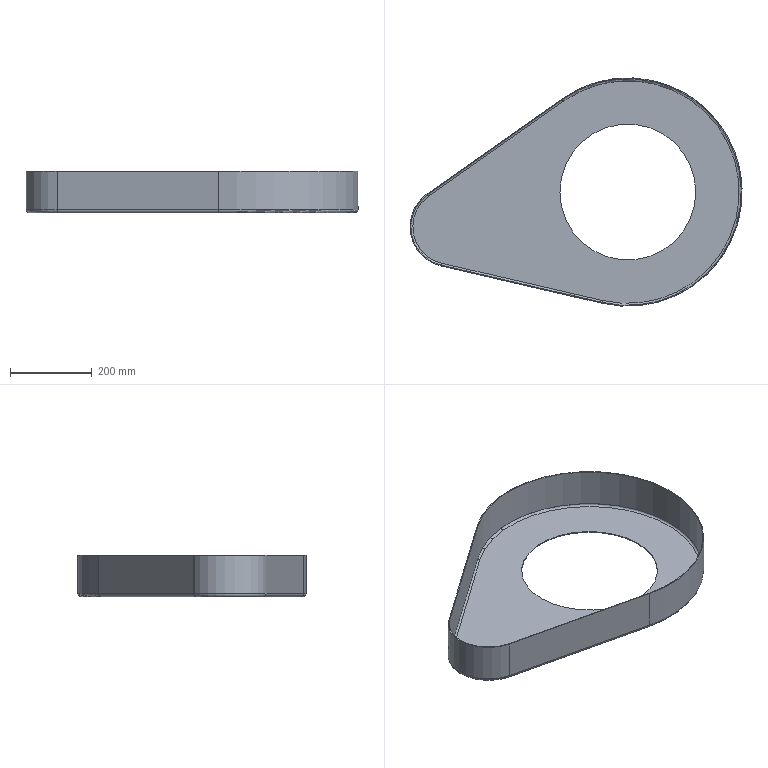Part | Creo | features DATUM PLANE 3, CURVE 2, PROTRUSION 2, ROUND 2, COORDINATE SYSTEM 1 | 1 solid | 21 faces | box 814.237 x 560 x 102 mm | volume 885224 mm3 | cylinder 10 | plane 7 | torus 4 | commonest cylinder face diameters 10 x2 14 x2 333.235 x2 193.453 x1 197.453 x1 556 x1
STEP:
#1=CARTESIAN_POINT('',(0.,0.,0.));
#2=DIRECTION('',(0.,0.,1.));
#3=DIRECTION('',(1.,0.,0.));
#4=AXIS2_PLACEMENT_3D('',#1,#2,#3);
#5=CARTESIAN_POINT('',(-50.882,-259.323,0.));
#6=VERTEX_POINT('',#5);
#7=CARTESIAN_POINT('',(-445.479,-167.904,0.));
#8=VERTEX_POINT('',#7);
#9=CARTESIAN_POINT('',(-50.882,-259.323,0.));
#10=DIRECTION('',(-0.9742,0.2257,0.));
#11=VECTOR('',#10,405.048);
#12=LINE('',#9,#11);
#13=EDGE_CURVE('',#6,#8,#12,.T.);
#14=ORIENTED_EDGE('',*,*,#13,.F.);
#15=CARTESIAN_POINT('',(-146.54,229.778,0.));
#16=VERTEX_POINT('',#15);
#17=CARTESIAN_POINT('',(10.734,6.632,0.));
#18=DIRECTION('',(0.,0.,-1.));
#19=DIRECTION('',(-0.5761,0.8174,0.));
#20=AXIS2_PLACEMENT_3D('',#17,#18,#19);
#21=CIRCLE('',#20,273.);
#22=EDGE_CURVE('',#16,#6,#21,.T.);
#23=ORIENTED_EDGE('',*,*,#22,.F.);
#24=CARTESIAN_POINT('',(-477.619,-3.568,0.));
#25=VERTEX_POINT('',#24);
#26=CARTESIAN_POINT('',(-477.619,-3.568,0.));
#27=DIRECTION('',(0.8174,0.5761,0.));
#28=VECTOR('',#27,405.048);
#29=LINE('',#26,#28);
#30=EDGE_CURVE('',#25,#16,#29,.T.);
#31=ORIENTED_EDGE('',*,*,#30,.F.);
#32=CARTESIAN_POINT('',(-424.776,-78.544,0.));
#33=DIRECTION('',(0.,0.,-1.));
#34=DIRECTION('',(-0.2257,-0.9742,0.));
#35=AXIS2_PLACEMENT_3D('',#32,#33,#34);
#36=CIRCLE('',#35,91.727);
#37=EDGE_CURVE('',#8,#25,#36,.T.);
#38=ORIENTED_EDGE('',*,*,#37,.F.);
#39=EDGE_LOOP('',(#14,#23,#31,#38));
#40=FACE_OUTER_BOUND('',#39,.F.);
#41=CARTESIAN_POINT('',(177.351,6.632,0.));
#42=VERTEX_POINT('',#41);
#43=CARTESIAN_POINT('',(-155.883,6.632,0.));
#44=VERTEX_POINT('',#43);
#45=CARTESIAN_POINT('',(10.734,6.632,0.));
#46=DIRECTION('',(0.,0.,-1.));
#47=DIRECTION('',(1.,0.,0.));
#48=AXIS2_PLACEMENT_3D('',#45,#46,#47);
#49=CIRCLE('',#48,166.617);
#50=EDGE_CURVE('',#42,#44,#49,.T.);
#51=ORIENTED_EDGE('',*,*,#50,.T.);
#52=CARTESIAN_POINT('',(10.734,6.632,0.));
#53=DIRECTION('',(0.,0.,-1.));
#54=DIRECTION('',(-1.,0.,0.));
#55=AXIS2_PLACEMENT_3D('',#52,#53,#54);
#56=CIRCLE('',#55,166.617);
#57=EDGE_CURVE('',#44,#42,#56,.T.);
#58=ORIENTED_EDGE('',*,*,#57,.T.);
#59=EDGE_LOOP('',(#51,#58));
#60=FACE_BOUND('',#59,.F.);
#61=CARTESIAN_POINT('',(0.,0.,0.));
#62=DIRECTION('',(0.,0.,1.));
#63=DIRECTION('',(1.,0.,0.));
#64=AXIS2_PLACEMENT_3D('',#61,#62,#63);
#65=PLANE('',#64);
#66=ADVANCED_FACE('',(#40,#60),#65,.F.);
#67=ORIENTED_EDGE('',*,*,#50,.F.);
#68=CARTESIAN_POINT('',(177.351,6.632,2.));
#69=VERTEX_POINT('',#68);
#70=CARTESIAN_POINT('',(177.351,6.632,0.));
#71=DIRECTION('',(0.,0.,1.));
#72=VECTOR('',#71,2.);
#73=LINE('',#70,#72);
#74=EDGE_CURVE('',#42,#69,#73,.T.);
#75=ORIENTED_EDGE('',*,*,#74,.T.);
#76=CARTESIAN_POINT('',(-155.883,6.632,2.));
#77=VERTEX_POINT('',#76);
#78=CARTESIAN_POINT('',(10.734,6.632,2.));
#79=DIRECTION('',(0.,0.,-1.));
#80=DIRECTION('',(1.,0.,0.));
#81=AXIS2_PLACEMENT_3D('',#78,#79,#80);
#82=CIRCLE('',#81,166.617);
#83=EDGE_CURVE('',#69,#77,#82,.T.);
#84=ORIENTED_EDGE('',*,*,#83,.T.);
#85=CARTESIAN_POINT('',(-155.883,6.632,0.));
#86=DIRECTION('',(0.,0.,1.));
#87=VECTOR('',#86,2.);
#88=LINE('',#85,#87);
#89=EDGE_CURVE('',#44,#77,#88,.T.);
#90=ORIENTED_EDGE('',*,*,#89,.F.);
#91=EDGE_LOOP('',(#67,#75,#84,#90));
#92=FACE_OUTER_BOUND('',#91,.F.);
#93=CARTESIAN_POINT('',(10.734,6.632,0.));
#94=DIRECTION('',(0.,0.,1.));
#95=DIRECTION('',(1.,0.,0.));
#96=AXIS2_PLACEMENT_3D('',#93,#94,#95);
#97=CYLINDRICAL_SURFACE('',#96,166.617);
#98=ADVANCED_FACE('',(#92),#97,.F.);
#99=ORIENTED_EDGE('',*,*,#57,.F.);
#100=ORIENTED_EDGE('',*,*,#89,.T.);
#101=CARTESIAN_POINT('',(10.734,6.632,2.));
#102=DIRECTION('',(0.,0.,-1.));
#103=DIRECTION('',(-1.,0.,0.));
#104=AXIS2_PLACEMENT_3D('',#101,#102,#103);
#105=CIRCLE('',#104,166.617);
#106=EDGE_CURVE('',#77,#69,#105,.T.);
#107=ORIENTED_EDGE('',*,*,#106,.T.);
#108=ORIENTED_EDGE('',*,*,#74,.F.);
#109=EDGE_LOOP('',(#99,#100,#107,#108));
#110=FACE_OUTER_BOUND('',#109,.F.);
#111=CARTESIAN_POINT('',(10.734,6.632,0.));
#112=DIRECTION('',(0.,0.,1.));
#113=DIRECTION('',(1.,0.,0.));
#114=AXIS2_PLACEMENT_3D('',#111,#112,#113);
#115=CYLINDRICAL_SURFACE('',#114,166.617);
#116=ADVANCED_FACE('',(#110),#115,.F.);
#117=CARTESIAN_POINT('',(-50.882,-259.323,2.));
#118=VERTEX_POINT('',#117);
#119=CARTESIAN_POINT('',(-445.479,-167.904,2.));
#120=VERTEX_POINT('',#119);
#121=CARTESIAN_POINT('',(-50.882,-259.323,2.));
#122=DIRECTION('',(-0.9742,0.2257,0.));
#123=VECTOR('',#122,405.048);
#124=LINE('',#121,#123);
#125=EDGE_CURVE('',#118,#120,#124,.T.);
#126=ORIENTED_EDGE('',*,*,#125,.T.);
#127=CARTESIAN_POINT('',(-477.619,-3.568,2.));
#128=VERTEX_POINT('',#127);
#129=CARTESIAN_POINT('',(-424.776,-78.544,2.));
#130=DIRECTION('',(0.,0.,-1.));
#131=DIRECTION('',(-0.2257,-0.9742,0.));
#132=AXIS2_PLACEMENT_3D('',#129,#130,#131);
#133=CIRCLE('',#132,91.727);
#134=EDGE_CURVE('',#120,#128,#133,.T.);
#135=ORIENTED_EDGE('',*,*,#134,.T.);
#136=CARTESIAN_POINT('',(-146.54,229.778,2.));
#137=VERTEX_POINT('',#136);
#138=CARTESIAN_POINT('',(-477.619,-3.568,2.));
#139=DIRECTION('',(0.8174,0.5761,0.));
#140=VECTOR('',#139,405.048);
#141=LINE('',#138,#140);
#142=EDGE_CURVE('',#128,#137,#141,.T.);
#143=ORIENTED_EDGE('',*,*,#142,.T.);
#144=CARTESIAN_POINT('',(10.734,6.632,2.));
#145=DIRECTION('',(0.,0.,-1.));
#146=DIRECTION('',(-0.5761,0.8174,0.));
#147=AXIS2_PLACEMENT_3D('',#144,#145,#146);
#148=CIRCLE('',#147,273.);
#149=EDGE_CURVE('',#137,#118,#148,.T.);
#150=ORIENTED_EDGE('',*,*,#149,.T.);
#151=EDGE_LOOP('',(#126,#135,#143,#150));
#152=FACE_OUTER_BOUND('',#151,.F.);
#153=ORIENTED_EDGE('',*,*,#83,.F.);
#154=ORIENTED_EDGE('',*,*,#106,.F.);
#155=EDGE_LOOP('',(#153,#154));
#156=FACE_BOUND('',#155,.F.);
#157=CARTESIAN_POINT('',(0.,0.,2.));
#158=DIRECTION('',(0.,0.,1.));
#159=DIRECTION('',(1.,0.,0.));
#160=AXIS2_PLACEMENT_3D('',#157,#158,#159);
#161=PLANE('',#160);
#162=ADVANCED_FACE('',(#152,#156),#161,.T.);
#163=ORIENTED_EDGE('',*,*,#125,.F.);
#164=CARTESIAN_POINT('',(-52.011,-264.194,7.));
#165=VERTEX_POINT('',#164);
#166=CARTESIAN_POINT('',(-50.882,-259.323,7.));
#167=DIRECTION('',(-0.9742,0.2257,0.));
#168=DIRECTION('',(0.,0.,-1.));
#169=AXIS2_PLACEMENT_3D('',#166,#167,#168);
#170=CIRCLE('',#169,5.);
#171=EDGE_CURVE('',#118,#165,#170,.T.);
#172=ORIENTED_EDGE('',*,*,#171,.T.);
#173=CARTESIAN_POINT('',(-446.607,-172.775,7.));
#174=VERTEX_POINT('',#173);
#175=CARTESIAN_POINT('',(-52.011,-264.194,7.));
#176=DIRECTION('',(-0.9742,0.2257,0.));
#177=VECTOR('',#176,405.048);
#178=LINE('',#175,#177);
#179=EDGE_CURVE('',#165,#174,#178,.T.);
#180=ORIENTED_EDGE('',*,*,#179,.T.);
#181=CARTESIAN_POINT('',(-445.479,-167.904,7.));
#182=DIRECTION('',(-0.9742,0.2257,0.));
#183=DIRECTION('',(0.,0.,-1.));
#184=AXIS2_PLACEMENT_3D('',#181,#182,#183);
#185=CIRCLE('',#184,5.);
#186=EDGE_CURVE('',#120,#174,#185,.T.);
#187=ORIENTED_EDGE('',*,*,#186,.F.);
#188=EDGE_LOOP('',(#163,#172,#180,#187));
#189=FACE_OUTER_BOUND('',#188,.F.);
#190=CARTESIAN_POINT('',(-49.393,-259.668,7.));
#191=DIRECTION('',(-0.9742,0.2257,0.));
#192=DIRECTION('',(0.,0.,-1.));
#193=AXIS2_PLACEMENT_3D('',#190,#191,#192);
#194=CYLINDRICAL_SURFACE('',#193,5.);
#195=ADVANCED_FACE('',(#189),#194,.F.);
#196=ORIENTED_EDGE('',*,*,#149,.F.);
#197=CARTESIAN_POINT('',(-149.42,233.865,7.));
#198=VERTEX_POINT('',#197);
#199=CARTESIAN_POINT('',(-146.54,229.778,7.));
#200=DIRECTION('',(0.8174,0.5761,0.));
#201=DIRECTION('',(0.,0.,-1.));
#202=AXIS2_PLACEMENT_3D('',#199,#200,#201);
#203=CIRCLE('',#202,5.);
#204=EDGE_CURVE('',#137,#198,#203,.T.);
#205=ORIENTED_EDGE('',*,*,#204,.T.);
#206=CARTESIAN_POINT('',(10.734,6.632,7.));
#207=DIRECTION('',(0.,0.,-1.));
#208=DIRECTION('',(-0.5761,0.8174,0.));
#209=AXIS2_PLACEMENT_3D('',#206,#207,#208);
#210=CIRCLE('',#209,278.);
#211=EDGE_CURVE('',#198,#165,#210,.T.);
#212=ORIENTED_EDGE('',*,*,#211,.T.);
#213=ORIENTED_EDGE('',*,*,#171,.F.);
#214=EDGE_LOOP('',(#196,#205,#212,#213));
#215=FACE_OUTER_BOUND('',#214,.F.);
#216=CARTESIAN_POINT('',(10.734,6.632,7.));
#217=DIRECTION('',(0.,0.,1.));
#218=DIRECTION('',(-0.5825,0.8129,0.));
#219=AXIS2_PLACEMENT_3D('',#216,#217,#218);
#220=TOROIDAL_SURFACE('',#219,273.,5.);
#221=ADVANCED_FACE('',(#215),#220,.F.);
#222=ORIENTED_EDGE('',*,*,#142,.F.);
#223=CARTESIAN_POINT('',(-480.5,0.5186,7.));
#224=VERTEX_POINT('',#223);
#225=CARTESIAN_POINT('',(-477.619,-3.568,7.));
#226=DIRECTION('',(0.8174,0.5761,0.));
#227=DIRECTION('',(0.,0.,-1.));
#228=AXIS2_PLACEMENT_3D('',#225,#226,#227);
#229=CIRCLE('',#228,5.);
#230=EDGE_CURVE('',#128,#224,#229,.T.);
#231=ORIENTED_EDGE('',*,*,#230,.T.);
#232=CARTESIAN_POINT('',(-480.5,0.5186,7.));
#233=DIRECTION('',(0.8174,0.5761,0.));
#234=VECTOR('',#233,405.048);
#235=LINE('',#232,#234);
#236=EDGE_CURVE('',#224,#198,#235,.T.);
#237=ORIENTED_EDGE('',*,*,#236,.T.);
#238=ORIENTED_EDGE('',*,*,#204,.F.);
#239=EDGE_LOOP('',(#222,#231,#237,#238));
#240=FACE_OUTER_BOUND('',#239,.F.);
#241=CARTESIAN_POINT('',(-478.868,-4.449,7.));
#242=DIRECTION('',(0.8174,0.5761,0.));
#243=DIRECTION('',(0.,0.,-1.));
#244=AXIS2_PLACEMENT_3D('',#241,#242,#243);
#245=CYLINDRICAL_SURFACE('',#244,5.);
#246=ADVANCED_FACE('',(#240),#245,.F.);
#247=ORIENTED_EDGE('',*,*,#134,.F.);
#248=ORIENTED_EDGE('',*,*,#186,.T.);
#249=CARTESIAN_POINT('',(-424.776,-78.544,7.));
#250=DIRECTION('',(0.,0.,-1.));
#251=DIRECTION('',(-0.2257,-0.9742,0.));
#252=AXIS2_PLACEMENT_3D('',#249,#250,#251);
#253=CIRCLE('',#252,96.727);
#254=EDGE_CURVE('',#174,#224,#253,.T.);
#255=ORIENTED_EDGE('',*,*,#254,.T.);
#256=ORIENTED_EDGE('',*,*,#230,.F.);
#257=EDGE_LOOP('',(#247,#248,#255,#256));
#258=FACE_OUTER_BOUND('',#257,.F.);
#259=CARTESIAN_POINT('',(-424.776,-78.544,7.));
#260=DIRECTION('',(0.,0.,1.));
#261=DIRECTION('',(-0.2038,-0.979,0.));
#262=AXIS2_PLACEMENT_3D('',#259,#260,#261);
#263=TOROIDAL_SURFACE('',#262,91.727,5.);
#264=ADVANCED_FACE('',(#258),#263,.F.);
#265=ORIENTED_EDGE('',*,*,#254,.F.);
#266=CARTESIAN_POINT('',(-446.607,-172.775,102.));
#267=VERTEX_POINT('',#266);
#268=CARTESIAN_POINT('',(-446.607,-172.775,7.));
#269=DIRECTION('',(0.,0.,1.));
#270=VECTOR('',#269,95.);
#271=LINE('',#268,#270);
#272=EDGE_CURVE('',#174,#267,#271,.T.);
#273=ORIENTED_EDGE('',*,*,#272,.T.);
#274=CARTESIAN_POINT('',(-480.5,0.5186,102.));
#275=VERTEX_POINT('',#274);
#276=CARTESIAN_POINT('',(-424.776,-78.544,102.));
#277=DIRECTION('',(0.,0.,-1.));
#278=DIRECTION('',(-0.2257,-0.9742,0.));
#279=AXIS2_PLACEMENT_3D('',#276,#277,#278);
#280=CIRCLE('',#279,96.727);
#281=EDGE_CURVE('',#267,#275,#280,.T.);
#282=ORIENTED_EDGE('',*,*,#281,.T.);
#283=CARTESIAN_POINT('',(-480.5,0.5186,7.));
#284=DIRECTION('',(0.,0.,1.));
#285=VECTOR('',#284,95.);
#286=LINE('',#283,#285);
#287=EDGE_CURVE('',#224,#275,#286,.T.);
#288=ORIENTED_EDGE('',*,*,#287,.F.);
#289=EDGE_LOOP('',(#265,#273,#282,#288));
#290=FACE_OUTER_BOUND('',#289,.F.);
#291=CARTESIAN_POINT('',(-424.776,-78.544,2.));
#292=DIRECTION('',(0.,0.,1.));
#293=DIRECTION('',(1.,0.,0.));
#294=AXIS2_PLACEMENT_3D('',#291,#292,#293);
#295=CYLINDRICAL_SURFACE('',#294,96.727);
#296=ADVANCED_FACE('',(#290),#295,.F.);
#297=ORIENTED_EDGE('',*,*,#179,.F.);
#298=CARTESIAN_POINT('',(-52.011,-264.194,102.));
#299=VERTEX_POINT('',#298);
#300=CARTESIAN_POINT('',(-52.011,-264.194,7.));
#301=DIRECTION('',(0.,0.,1.));
#302=VECTOR('',#301,95.);
#303=LINE('',#300,#302);
#304=EDGE_CURVE('',#165,#299,#303,.T.);
#305=ORIENTED_EDGE('',*,*,#304,.T.);
#306=CARTESIAN_POINT('',(-52.011,-264.194,102.));
#307=DIRECTION('',(-0.9742,0.2257,0.));
#308=VECTOR('',#307,405.048);
#309=LINE('',#306,#308);
#310=EDGE_CURVE('',#299,#267,#309,.T.);
#311=ORIENTED_EDGE('',*,*,#310,.T.);
#312=ORIENTED_EDGE('',*,*,#272,.F.);
#313=EDGE_LOOP('',(#297,#305,#311,#312));
#314=FACE_OUTER_BOUND('',#313,.F.);
#315=CARTESIAN_POINT('',(-52.011,-264.194,2.));
#316=DIRECTION('',(0.2257,0.9742,0.));
#317=DIRECTION('',(-0.9742,0.2257,0.));
#318=AXIS2_PLACEMENT_3D('',#315,#316,#317);
#319=PLANE('',#318);
#320=ADVANCED_FACE('',(#314),#319,.T.);
#321=ORIENTED_EDGE('',*,*,#211,.F.);
#322=CARTESIAN_POINT('',(-149.42,233.865,102.));
#323=VERTEX_POINT('',#322);
#324=CARTESIAN_POINT('',(-149.42,233.865,7.));
#325=DIRECTION('',(0.,0.,1.));
#326=VECTOR('',#325,95.);
#327=LINE('',#324,#326);
#328=EDGE_CURVE('',#198,#323,#327,.T.);
#329=ORIENTED_EDGE('',*,*,#328,.T.);
#330=CARTESIAN_POINT('',(10.734,6.632,102.));
#331=DIRECTION('',(0.,0.,-1.));
#332=DIRECTION('',(-0.5761,0.8174,0.));
#333=AXIS2_PLACEMENT_3D('',#330,#331,#332);
#334=CIRCLE('',#333,278.);
#335=EDGE_CURVE('',#323,#299,#334,.T.);
#336=ORIENTED_EDGE('',*,*,#335,.T.);
#337=ORIENTED_EDGE('',*,*,#304,.F.);
#338=EDGE_LOOP('',(#321,#329,#336,#337));
#339=FACE_OUTER_BOUND('',#338,.F.);
#340=CARTESIAN_POINT('',(10.734,6.632,2.));
#341=DIRECTION('',(0.,0.,1.));
#342=DIRECTION('',(1.,0.,0.));
#343=AXIS2_PLACEMENT_3D('',#340,#341,#342);
#344=CYLINDRICAL_SURFACE('',#343,278.);
#345=ADVANCED_FACE('',(#339),#344,.F.);
#346=ORIENTED_EDGE('',*,*,#236,.F.);
#347=ORIENTED_EDGE('',*,*,#287,.T.);
#348=CARTESIAN_POINT('',(-480.5,0.5186,102.));
#349=DIRECTION('',(0.8174,0.5761,0.));
#350=VECTOR('',#349,405.048);
#351=LINE('',#348,#350);
#352=EDGE_CURVE('',#275,#323,#351,.T.);
#353=ORIENTED_EDGE('',*,*,#352,.T.);
#354=ORIENTED_EDGE('',*,*,#328,.F.);
#355=EDGE_LOOP('',(#346,#347,#353,#354));
#356=FACE_OUTER_BOUND('',#355,.F.);
#357=CARTESIAN_POINT('',(-480.5,0.5186,2.));
#358=DIRECTION('',(0.5761,-0.8174,0.));
#359=DIRECTION('',(0.8174,0.5761,0.));
#360=AXIS2_PLACEMENT_3D('',#357,#358,#359);
#361=PLANE('',#360);
#362=ADVANCED_FACE('',(#356),#361,.T.);
#363=CARTESIAN_POINT('',(-52.462,-266.143,102.));
#364=VERTEX_POINT('',#363);
#365=CARTESIAN_POINT('',(-150.573,235.5,102.));
#366=VERTEX_POINT('',#365);
#367=CARTESIAN_POINT('',(10.734,6.632,102.));
#368=DIRECTION('',(0.,0.,1.));
#369=DIRECTION('',(-0.2257,-0.9742,0.));
#370=AXIS2_PLACEMENT_3D('',#367,#368,#369);
#371=CIRCLE('',#370,280.);
#372=EDGE_CURVE('',#364,#366,#371,.T.);
#373=ORIENTED_EDGE('',*,*,#372,.F.);
#374=CARTESIAN_POINT('',(-447.058,-174.723,102.));
#375=VERTEX_POINT('',#374);
#376=CARTESIAN_POINT('',(-447.058,-174.723,102.));
#377=DIRECTION('',(0.9742,-0.2257,0.));
#378=VECTOR('',#377,405.048);
#379=LINE('',#376,#378);
#380=EDGE_CURVE('',#375,#364,#379,.T.);
#381=ORIENTED_EDGE('',*,*,#380,.F.);
#382=CARTESIAN_POINT('',(-481.652,2.153,102.));
#383=VERTEX_POINT('',#382);
#384=CARTESIAN_POINT('',(-424.776,-78.544,102.));
#385=DIRECTION('',(0.,0.,1.));
#386=DIRECTION('',(-0.5761,0.8174,0.));
#387=AXIS2_PLACEMENT_3D('',#384,#385,#386);
#388=CIRCLE('',#387,98.727);
#389=EDGE_CURVE('',#383,#375,#388,.T.);
#390=ORIENTED_EDGE('',*,*,#389,.F.);
#391=CARTESIAN_POINT('',(-150.573,235.5,102.));
#392=DIRECTION('',(-0.8174,-0.5761,0.));
#393=VECTOR('',#392,405.048);
#394=LINE('',#391,#393);
#395=EDGE_CURVE('',#366,#383,#394,.T.);
#396=ORIENTED_EDGE('',*,*,#395,.F.);
#397=EDGE_LOOP('',(#373,#381,#390,#396));
#398=FACE_OUTER_BOUND('',#397,.F.);
#399=ORIENTED_EDGE('',*,*,#310,.F.);
#400=ORIENTED_EDGE('',*,*,#335,.F.);
#401=ORIENTED_EDGE('',*,*,#352,.F.);
#402=ORIENTED_EDGE('',*,*,#281,.F.);
#403=EDGE_LOOP('',(#399,#400,#401,#402));
#404=FACE_BOUND('',#403,.F.);
#405=CARTESIAN_POINT('',(0.,0.,102.));
#406=DIRECTION('',(0.,0.,1.));
#407=DIRECTION('',(1.,0.,0.));
#408=AXIS2_PLACEMENT_3D('',#405,#406,#407);
#409=PLANE('',#408);
#410=ADVANCED_FACE('',(#398,#404),#409,.T.);
#411=CARTESIAN_POINT('',(-150.573,235.5,7.));
#412=VERTEX_POINT('',#411);
#413=CARTESIAN_POINT('',(-52.462,-266.143,7.));
#414=VERTEX_POINT('',#413);
#415=CARTESIAN_POINT('',(10.734,6.632,7.));
#416=DIRECTION('',(0.,0.,-1.));
#417=DIRECTION('',(-0.5761,0.8174,0.));
#418=AXIS2_PLACEMENT_3D('',#415,#416,#417);
#419=CIRCLE('',#418,280.);
#420=EDGE_CURVE('',#412,#414,#419,.T.);
#421=ORIENTED_EDGE('',*,*,#420,.T.);
#422=CARTESIAN_POINT('',(-52.462,-266.143,102.));
#423=DIRECTION('',(0.,0.,-1.));
#424=VECTOR('',#423,95.);
#425=LINE('',#422,#424);
#426=EDGE_CURVE('',#364,#414,#425,.T.);
#427=ORIENTED_EDGE('',*,*,#426,.F.);
#428=ORIENTED_EDGE('',*,*,#372,.T.);
#429=CARTESIAN_POINT('',(-150.573,235.5,7.));
#430=DIRECTION('',(0.,0.,1.));
#431=VECTOR('',#430,95.);
#432=LINE('',#429,#431);
#433=EDGE_CURVE('',#412,#366,#432,.T.);
#434=ORIENTED_EDGE('',*,*,#433,.F.);
#435=EDGE_LOOP('',(#421,#427,#428,#434));
#436=FACE_OUTER_BOUND('',#435,.F.);
#437=CARTESIAN_POINT('',(10.734,6.632,0.));
#438=DIRECTION('',(0.,0.,1.));
#439=DIRECTION('',(1.,0.,0.));
#440=AXIS2_PLACEMENT_3D('',#437,#438,#439);
#441=CYLINDRICAL_SURFACE('',#440,280.);
#442=ADVANCED_FACE('',(#436),#441,.T.);
#443=ORIENTED_EDGE('',*,*,#22,.T.);
#444=CARTESIAN_POINT('',(-50.882,-259.323,7.));
#445=DIRECTION('',(-0.9742,0.2257,0.));
#446=DIRECTION('',(0.,0.,-1.));
#447=AXIS2_PLACEMENT_3D('',#444,#445,#446);
#448=CIRCLE('',#447,7.);
#449=EDGE_CURVE('',#6,#414,#448,.T.);
#450=ORIENTED_EDGE('',*,*,#449,.T.);
#451=ORIENTED_EDGE('',*,*,#420,.F.);
#452=CARTESIAN_POINT('',(-146.54,229.778,7.));
#453=DIRECTION('',(0.8174,0.5761,0.));
#454=DIRECTION('',(0.,0.,-1.));
#455=AXIS2_PLACEMENT_3D('',#452,#453,#454);
#456=CIRCLE('',#455,7.);
#457=EDGE_CURVE('',#16,#412,#456,.T.);
#458=ORIENTED_EDGE('',*,*,#457,.F.);
#459=EDGE_LOOP('',(#443,#450,#451,#458));
#460=FACE_OUTER_BOUND('',#459,.F.);
#461=CARTESIAN_POINT('',(10.734,6.632,7.));
#462=DIRECTION('',(0.,0.,1.));
#463=DIRECTION('',(-0.5824,0.8129,0.));
#464=AXIS2_PLACEMENT_3D('',#461,#462,#463);
#465=TOROIDAL_SURFACE('',#464,273.,7.);
#466=ADVANCED_FACE('',(#460),#465,.T.);
#467=ORIENTED_EDGE('',*,*,#13,.T.);
#468=CARTESIAN_POINT('',(-447.058,-174.723,7.));
#469=VERTEX_POINT('',#468);
#470=CARTESIAN_POINT('',(-445.479,-167.904,7.));
#471=DIRECTION('',(-0.9742,0.2257,0.));
#472=DIRECTION('',(0.,0.,-1.));
#473=AXIS2_PLACEMENT_3D('',#470,#471,#472);
#474=CIRCLE('',#473,7.);
#475=EDGE_CURVE('',#8,#469,#474,.T.);
#476=ORIENTED_EDGE('',*,*,#475,.T.);
#477=CARTESIAN_POINT('',(-52.462,-266.143,7.));
#478=DIRECTION('',(-0.9742,0.2257,0.));
#479=VECTOR('',#478,405.048);
#480=LINE('',#477,#479);
#481=EDGE_CURVE('',#414,#469,#480,.T.);
#482=ORIENTED_EDGE('',*,*,#481,.F.);
#483=ORIENTED_EDGE('',*,*,#449,.F.);
#484=EDGE_LOOP('',(#467,#476,#482,#483));
#485=FACE_OUTER_BOUND('',#484,.F.);
#486=CARTESIAN_POINT('',(-48.767,-259.813,7.));
#487=DIRECTION('',(-0.9742,0.2257,0.));
#488=DIRECTION('',(0.,0.,-1.));
#489=AXIS2_PLACEMENT_3D('',#486,#487,#488);
#490=CYLINDRICAL_SURFACE('',#489,7.);
#491=ADVANCED_FACE('',(#485),#490,.T.);
#492=ORIENTED_EDGE('',*,*,#37,.T.);
#493=CARTESIAN_POINT('',(-481.652,2.153,7.));
#494=VERTEX_POINT('',#493);
#495=CARTESIAN_POINT('',(-477.619,-3.568,7.));
#496=DIRECTION('',(0.8174,0.5761,0.));
#497=DIRECTION('',(0.,0.,-1.));
#498=AXIS2_PLACEMENT_3D('',#495,#496,#497);
#499=CIRCLE('',#498,7.);
#500=EDGE_CURVE('',#25,#494,#499,.T.);
#501=ORIENTED_EDGE('',*,*,#500,.T.);
#502=CARTESIAN_POINT('',(-424.776,-78.544,7.));
#503=DIRECTION('',(0.,0.,-1.));
#504=DIRECTION('',(-0.2257,-0.9742,0.));
#505=AXIS2_PLACEMENT_3D('',#502,#503,#504);
#506=CIRCLE('',#505,98.727);
#507=EDGE_CURVE('',#469,#494,#506,.T.);
#508=ORIENTED_EDGE('',*,*,#507,.F.);
#509=ORIENTED_EDGE('',*,*,#475,.F.);
#510=EDGE_LOOP('',(#492,#501,#508,#509));
#511=FACE_OUTER_BOUND('',#510,.F.);
#512=CARTESIAN_POINT('',(-424.776,-78.544,7.));
#513=DIRECTION('',(0.,0.,1.));
#514=DIRECTION('',(-0.2042,-0.9789,0.));
#515=AXIS2_PLACEMENT_3D('',#512,#513,#514);
#516=TOROIDAL_SURFACE('',#515,91.727,7.);
#517=ADVANCED_FACE('',(#511),#516,.T.);
#518=ORIENTED_EDGE('',*,*,#30,.T.);
#519=ORIENTED_EDGE('',*,*,#457,.T.);
#520=CARTESIAN_POINT('',(-481.652,2.153,7.));
#521=DIRECTION('',(0.8174,0.5761,0.));
#522=VECTOR('',#521,405.048);
#523=LINE('',#520,#522);
#524=EDGE_CURVE('',#494,#412,#523,.T.);
#525=ORIENTED_EDGE('',*,*,#524,.F.);
#526=ORIENTED_EDGE('',*,*,#500,.F.);
#527=EDGE_LOOP('',(#518,#519,#525,#526));
#528=FACE_OUTER_BOUND('',#527,.F.);
#529=CARTESIAN_POINT('',(-479.393,-4.819,7.));
#530=DIRECTION('',(0.8174,0.5761,0.));
#531=DIRECTION('',(0.,0.,-1.));
#532=AXIS2_PLACEMENT_3D('',#529,#530,#531);
#533=CYLINDRICAL_SURFACE('',#532,7.);
#534=ADVANCED_FACE('',(#528),#533,.T.);
#535=ORIENTED_EDGE('',*,*,#524,.T.);
#536=ORIENTED_EDGE('',*,*,#433,.T.);
#537=ORIENTED_EDGE('',*,*,#395,.T.);
#538=CARTESIAN_POINT('',(-481.652,2.153,7.));
#539=DIRECTION('',(0.,0.,1.));
#540=VECTOR('',#539,95.);
#541=LINE('',#538,#540);
#542=EDGE_CURVE('',#494,#383,#541,.T.);
#543=ORIENTED_EDGE('',*,*,#542,.F.);
#544=EDGE_LOOP('',(#535,#536,#537,#543));
#545=FACE_OUTER_BOUND('',#544,.F.);
#546=CARTESIAN_POINT('',(-150.573,235.5,0.));
#547=DIRECTION('',(-0.5761,0.8174,0.));
#548=DIRECTION('',(-0.8174,-0.5761,0.));
#549=AXIS2_PLACEMENT_3D('',#546,#547,#548);
#550=PLANE('',#549);
#551=ADVANCED_FACE('',(#545),#550,.T.);
#552=ORIENTED_EDGE('',*,*,#507,.T.);
#553=ORIENTED_EDGE('',*,*,#542,.T.);
#554=ORIENTED_EDGE('',*,*,#389,.T.);
#555=CARTESIAN_POINT('',(-447.058,-174.723,7.));
#556=DIRECTION('',(0.,0.,1.));
#557=VECTOR('',#556,95.);
#558=LINE('',#555,#557);
#559=EDGE_CURVE('',#469,#375,#558,.T.);
#560=ORIENTED_EDGE('',*,*,#559,.F.);
#561=EDGE_LOOP('',(#552,#553,#554,#560));
#562=FACE_OUTER_BOUND('',#561,.F.);
#563=CARTESIAN_POINT('',(-424.776,-78.544,0.));
#564=DIRECTION('',(0.,0.,1.));
#565=DIRECTION('',(1.,0.,0.));
#566=AXIS2_PLACEMENT_3D('',#563,#564,#565);
#567=CYLINDRICAL_SURFACE('',#566,98.727);
#568=ADVANCED_FACE('',(#562),#567,.T.);
#569=ORIENTED_EDGE('',*,*,#481,.T.);
#570=ORIENTED_EDGE('',*,*,#559,.T.);
#571=ORIENTED_EDGE('',*,*,#380,.T.);
#572=ORIENTED_EDGE('',*,*,#426,.T.);
#573=EDGE_LOOP('',(#569,#570,#571,#572));
#574=FACE_OUTER_BOUND('',#573,.F.);
#575=CARTESIAN_POINT('',(-447.058,-174.723,0.));
#576=DIRECTION('',(-0.2257,-0.9742,0.));
#577=DIRECTION('',(0.9742,-0.2257,0.));
#578=AXIS2_PLACEMENT_3D('',#575,#576,#577);
#579=PLANE('',#578);
#580=ADVANCED_FACE('',(#574),#579,.T.);
#581=CLOSED_SHELL('',(#66,#98,#116,#162,#195,#221,#246,#264,#296,#320,#345,#362,#410,#442,#466,#491,#517,#534,#551,#568,#580));
#582=MANIFOLD_SOLID_BREP('',#581);
#583=(LENGTH_UNIT()NAMED_UNIT(*)SI_UNIT(.MILLI.,.METRE.));
#584=UNCERTAINTY_MEASURE_WITH_UNIT(LENGTH_MEASURE(0.09937),#583,'','');
#585=(NAMED_UNIT(*)PLANE_ANGLE_UNIT()SI_UNIT($,.RADIAN.));
#586=PLANE_ANGLE_MEASURE_WITH_UNIT(PLANE_ANGLE_MEASURE(0.01745),#585);
#587=(CONVERSION_BASED_UNIT('DEGREE',#586)NAMED_UNIT(*)PLANE_ANGLE_UNIT());
#588=(NAMED_UNIT(*)SI_UNIT($,.STERADIAN.)SOLID_ANGLE_UNIT());
#589=(GEOMETRIC_REPRESENTATION_CONTEXT(3)GLOBAL_UNCERTAINTY_ASSIGNED_CONTEXT((#584))GLOBAL_UNIT_ASSIGNED_CONTEXT((#583,#587,#588))REPRESENTATION_CONTEXT('',''));
#590=ADVANCED_BREP_SHAPE_REPRESENTATION('',(#4,#582),#589);